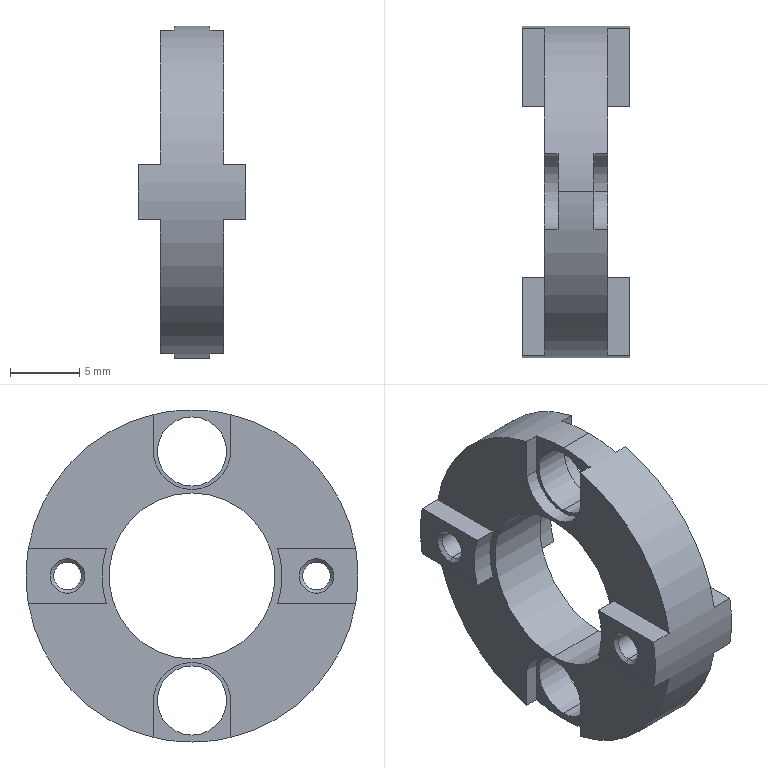Part | STEP file | _DBA11-D25-d10-e12-004.stp | 1 solid | 56 faces | box 7.8 x 24 x 24 mm | volume 1439 mm3 | plane 26 | cylinder 22 | cone 8 | commonest cylinder face diameters 5.58 x6 2.013 x4 5 x4 13 x4 12 x2 24 x2